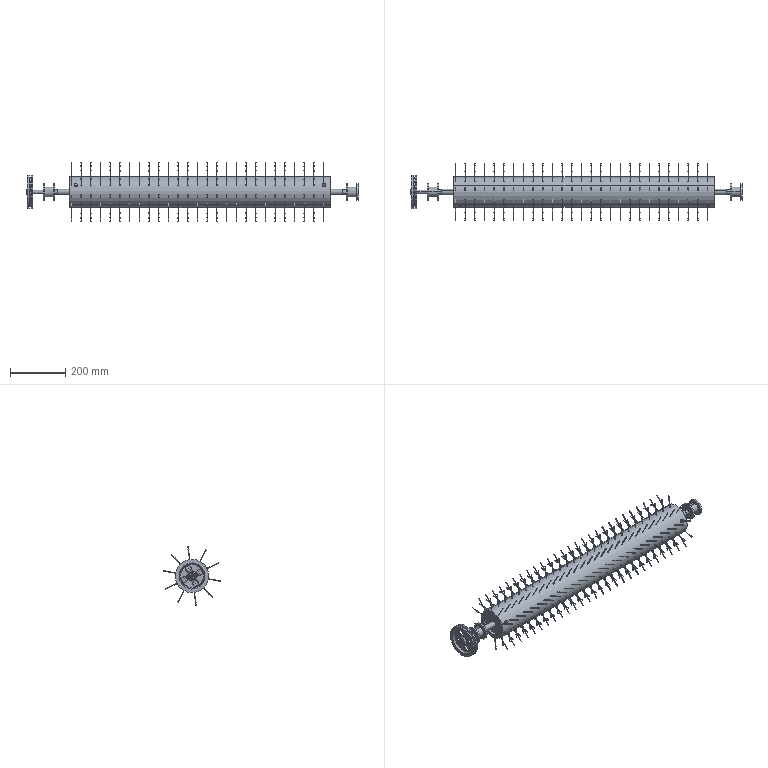Part | NX | features BREP 291 | 310 solids | 1452 faces | box 1198 x 209.075 x 210.255 mm | volume 5412337 mm3 | cylinder 747 | plane 675 | cone 22 | torus 8 | commonest cylinder face diameters 2 x538 6 x74 8 x32 12 x14 15 x12 19 x8